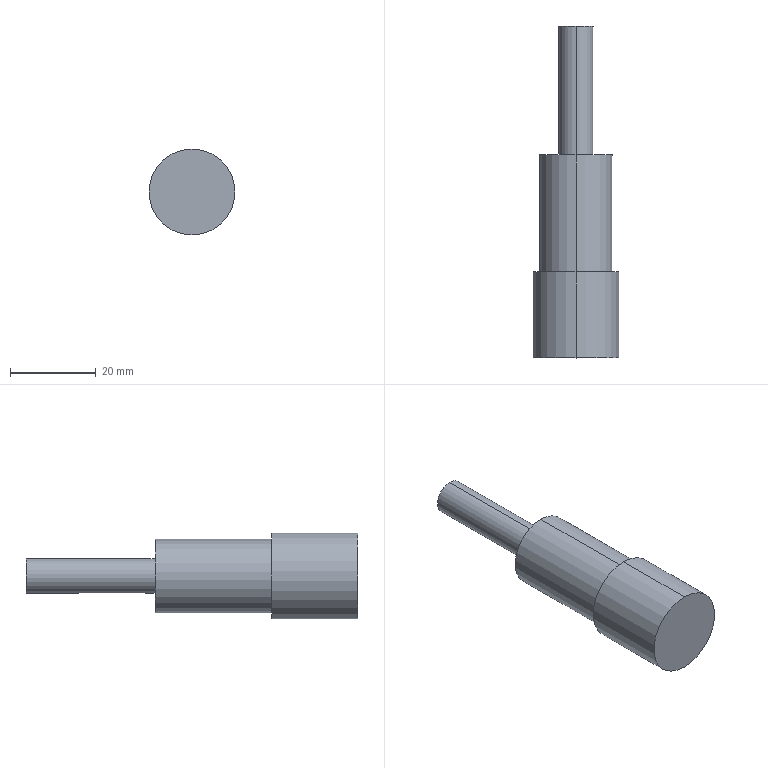Part | SolidWorks | features ICE 3, Extrusion 1 | 1 solid | 15 faces | box 20 x 77.2 x 20 mm | volume 13929 mm3 | cylinder 8 | plane 7 | commonest cylinder face diameters 2 x2 8 x2 17 x2 20 x2
STEP:
#1=CARTESIAN_POINT('',(0.,77.2,4.));
#2=VERTEX_POINT('',#1);
#3=CARTESIAN_POINT('',(0.,77.2,-4.));
#4=VERTEX_POINT('',#3);
#5=CARTESIAN_POINT('',(0.,77.2,0.));
#6=DIRECTION('',(0.,1.,0.));
#7=DIRECTION('',(0.,0.,1.));
#8=AXIS2_PLACEMENT_3D('',#5,#6,#7);
#9=CIRCLE('',#8,4.);
#10=EDGE_CURVE('',#2,#4,#9,.T.);
#11=ORIENTED_EDGE('',*,*,#10,.F.);
#12=CARTESIAN_POINT('',(0.,47.2,4.));
#13=VERTEX_POINT('',#12);
#14=CARTESIAN_POINT('',(0.,77.2,4.));
#15=DIRECTION('',(0.,-1.,0.));
#16=VECTOR('',#15,1000.);
#17=LINE('',#14,#16);
#18=EDGE_CURVE('',#2,#13,#17,.T.);
#19=ORIENTED_EDGE('',*,*,#18,.T.);
#20=CARTESIAN_POINT('',(0.,47.2,-4.));
#21=VERTEX_POINT('',#20);
#22=CARTESIAN_POINT('',(0.,47.2,0.));
#23=DIRECTION('',(0.,1.,0.));
#24=DIRECTION('',(0.,0.,1.));
#25=AXIS2_PLACEMENT_3D('',#22,#23,#24);
#26=CIRCLE('',#25,4.);
#27=EDGE_CURVE('',#13,#21,#26,.T.);
#28=ORIENTED_EDGE('',*,*,#27,.T.);
#29=CARTESIAN_POINT('',(0.,49.2,-4.));
#30=VERTEX_POINT('',#29);
#31=CARTESIAN_POINT('',(0.,77.2,-4.));
#32=DIRECTION('',(0.,-1.,0.));
#33=VECTOR('',#32,1000.);
#34=LINE('',#31,#33);
#35=EDGE_CURVE('',#30,#21,#34,.T.);
#36=ORIENTED_EDGE('',*,*,#35,.F.);
#37=CARTESIAN_POINT('',(1.,50.2,-3.873));
#38=VERTEX_POINT('',#37);
#39=CARTESIAN_POINT('',(0.,49.2,-4.));
#40=CARTESIAN_POINT('',(0.1309,49.2,-4.));
#41=CARTESIAN_POINT('',(0.2621,49.226,-3.993));
#42=CARTESIAN_POINT('',(0.5047,49.327,-3.97));
#43=CARTESIAN_POINT('',(0.6146,49.4,-3.954));
#44=CARTESIAN_POINT('',(0.7997,49.585,-3.92));
#45=CARTESIAN_POINT('',(0.8733,49.696,-3.904));
#46=CARTESIAN_POINT('',(0.9735,49.937,-3.88));
#47=CARTESIAN_POINT('',(1.,50.067,-3.873));
#48=CARTESIAN_POINT('',(1.,50.2,-3.873));
#49=B_SPLINE_CURVE_WITH_KNOTS('',3,(#39,#40,#41,#42,#43,#44,#45,#46,#47,#48),.UNSPECIFIED.,.F.,.F.,(4,2,2,2,4),(0.00157,0.001962,0.002354,0.002746,0.003138),.UNSPECIFIED.);
#50=EDGE_CURVE('',#30,#38,#49,.T.);
#51=ORIENTED_EDGE('',*,*,#50,.T.);
#52=CARTESIAN_POINT('',(1.,64.2,-3.873));
#53=VERTEX_POINT('',#52);
#54=CARTESIAN_POINT('',(1.,77.2,-3.873));
#55=DIRECTION('',(0.,1.,0.));
#56=VECTOR('',#55,1000.);
#57=LINE('',#54,#56);
#58=EDGE_CURVE('',#38,#53,#57,.T.);
#59=ORIENTED_EDGE('',*,*,#58,.T.);
#60=CARTESIAN_POINT('',(0.,65.2,-4.));
#61=VERTEX_POINT('',#60);
#62=CARTESIAN_POINT('',(1.,64.2,-3.873));
#63=CARTESIAN_POINT('',(1.,64.333,-3.873));
#64=CARTESIAN_POINT('',(0.9737,64.463,-3.88));
#65=CARTESIAN_POINT('',(0.873,64.705,-3.904));
#66=CARTESIAN_POINT('',(0.7987,64.816,-3.921));
#67=CARTESIAN_POINT('',(0.6149,64.999,-3.954));
#68=CARTESIAN_POINT('',(0.5037,65.074,-3.97));
#69=CARTESIAN_POINT('',(0.2631,65.174,-3.993));
#70=CARTESIAN_POINT('',(0.1311,65.2,-4.));
#71=CARTESIAN_POINT('',(0.,65.2,-4.));
#72=B_SPLINE_CURVE_WITH_KNOTS('',3,(#62,#63,#64,#65,#66,#67,#68,#69,#70,#71),.UNSPECIFIED.,.F.,.F.,(4,2,2,2,4),(0.,0.0003925,0.0007849,0.001177,0.00157),.UNSPECIFIED.);
#73=EDGE_CURVE('',#53,#61,#72,.T.);
#74=ORIENTED_EDGE('',*,*,#73,.T.);
#75=CARTESIAN_POINT('',(0.,77.2,-4.));
#76=DIRECTION('',(0.,-1.,0.));
#77=VECTOR('',#76,1000.);
#78=LINE('',#75,#77);
#79=EDGE_CURVE('',#4,#61,#78,.T.);
#80=ORIENTED_EDGE('',*,*,#79,.F.);
#81=EDGE_LOOP('',(#11,#19,#28,#36,#51,#59,#74,#80));
#82=FACE_OUTER_BOUND('',#81,.T.);
#83=CARTESIAN_POINT('',(0.,77.2,0.));
#84=DIRECTION('',(0.,-1.,0.));
#85=DIRECTION('',(0.,0.,-1.));
#86=AXIS2_PLACEMENT_3D('',#83,#84,#85);
#87=CYLINDRICAL_SURFACE('',#86,4.);
#88=ADVANCED_FACE('',(#82),#87,.T.);
#89=CARTESIAN_POINT('',(0.,47.2,8.5));
#90=VERTEX_POINT('',#89);
#91=CARTESIAN_POINT('',(0.,47.2,-8.5));
#92=VERTEX_POINT('',#91);
#93=CARTESIAN_POINT('',(0.,47.2,0.));
#94=DIRECTION('',(0.,1.,0.));
#95=DIRECTION('',(0.,0.,1.));
#96=AXIS2_PLACEMENT_3D('',#93,#94,#95);
#97=CIRCLE('',#96,8.5);
#98=EDGE_CURVE('',#90,#92,#97,.T.);
#99=ORIENTED_EDGE('',*,*,#98,.F.);
#100=CARTESIAN_POINT('',(0.,20.,8.5));
#101=VERTEX_POINT('',#100);
#102=CARTESIAN_POINT('',(0.,47.2,8.5));
#103=DIRECTION('',(0.,-1.,0.));
#104=VECTOR('',#103,1000.);
#105=LINE('',#102,#104);
#106=EDGE_CURVE('',#90,#101,#105,.T.);
#107=ORIENTED_EDGE('',*,*,#106,.T.);
#108=CARTESIAN_POINT('',(0.,20.,-8.5));
#109=VERTEX_POINT('',#108);
#110=CARTESIAN_POINT('',(0.,20.,0.));
#111=DIRECTION('',(0.,1.,0.));
#112=DIRECTION('',(0.,0.,1.));
#113=AXIS2_PLACEMENT_3D('',#110,#111,#112);
#114=CIRCLE('',#113,8.5);
#115=EDGE_CURVE('',#101,#109,#114,.T.);
#116=ORIENTED_EDGE('',*,*,#115,.T.);
#117=CARTESIAN_POINT('',(0.,47.2,-8.5));
#118=DIRECTION('',(0.,-1.,0.));
#119=VECTOR('',#118,1000.);
#120=LINE('',#117,#119);
#121=EDGE_CURVE('',#92,#109,#120,.T.);
#122=ORIENTED_EDGE('',*,*,#121,.F.);
#123=EDGE_LOOP('',(#99,#107,#116,#122));
#124=FACE_OUTER_BOUND('',#123,.T.);
#125=CARTESIAN_POINT('',(0.,47.2,0.));
#126=DIRECTION('',(0.,-1.,0.));
#127=DIRECTION('',(0.,0.,-1.));
#128=AXIS2_PLACEMENT_3D('',#125,#126,#127);
#129=CYLINDRICAL_SURFACE('',#128,8.5);
#130=ADVANCED_FACE('',(#124),#129,.T.);
#131=CARTESIAN_POINT('',(0.,20.,10.));
#132=VERTEX_POINT('',#131);
#133=CARTESIAN_POINT('',(0.,20.,-10.));
#134=VERTEX_POINT('',#133);
#135=CARTESIAN_POINT('',(0.,20.,0.));
#136=DIRECTION('',(0.,1.,0.));
#137=DIRECTION('',(0.,0.,1.));
#138=AXIS2_PLACEMENT_3D('',#135,#136,#137);
#139=CIRCLE('',#138,10.);
#140=EDGE_CURVE('',#132,#134,#139,.T.);
#141=ORIENTED_EDGE('',*,*,#140,.F.);
#142=CARTESIAN_POINT('',(0.,0.,10.));
#143=VERTEX_POINT('',#142);
#144=CARTESIAN_POINT('',(0.,20.,10.));
#145=DIRECTION('',(0.,-1.,0.));
#146=VECTOR('',#145,1000.);
#147=LINE('',#144,#146);
#148=EDGE_CURVE('',#132,#143,#147,.T.);
#149=ORIENTED_EDGE('',*,*,#148,.T.);
#150=CARTESIAN_POINT('',(0.,0.,-10.));
#151=VERTEX_POINT('',#150);
#152=CARTESIAN_POINT('',(0.,0.,0.));
#153=DIRECTION('',(0.,1.,0.));
#154=DIRECTION('',(0.,0.,1.));
#155=AXIS2_PLACEMENT_3D('',#152,#153,#154);
#156=CIRCLE('',#155,10.);
#157=EDGE_CURVE('',#143,#151,#156,.T.);
#158=ORIENTED_EDGE('',*,*,#157,.T.);
#159=CARTESIAN_POINT('',(0.,20.,-10.));
#160=DIRECTION('',(0.,-1.,0.));
#161=VECTOR('',#160,1000.);
#162=LINE('',#159,#161);
#163=EDGE_CURVE('',#134,#151,#162,.T.);
#164=ORIENTED_EDGE('',*,*,#163,.F.);
#165=EDGE_LOOP('',(#141,#149,#158,#164));
#166=FACE_OUTER_BOUND('',#165,.T.);
#167=CARTESIAN_POINT('',(0.,20.,0.));
#168=DIRECTION('',(0.,-1.,0.));
#169=DIRECTION('',(0.,0.,-1.));
#170=AXIS2_PLACEMENT_3D('',#167,#168,#169);
#171=CYLINDRICAL_SURFACE('',#170,10.);
#172=ADVANCED_FACE('',(#166),#171,.T.);
#173=ORIENTED_EDGE('',*,*,#148,.F.);
#174=CARTESIAN_POINT('',(0.,20.,0.));
#175=DIRECTION('',(0.,1.,0.));
#176=DIRECTION('',(0.,0.,1.));
#177=AXIS2_PLACEMENT_3D('',#174,#175,#176);
#178=CIRCLE('',#177,10.);
#179=EDGE_CURVE('',#134,#132,#178,.T.);
#180=ORIENTED_EDGE('',*,*,#179,.F.);
#181=ORIENTED_EDGE('',*,*,#163,.T.);
#182=CARTESIAN_POINT('',(0.,0.,0.));
#183=DIRECTION('',(0.,1.,0.));
#184=DIRECTION('',(0.,0.,1.));
#185=AXIS2_PLACEMENT_3D('',#182,#183,#184);
#186=CIRCLE('',#185,10.);
#187=EDGE_CURVE('',#151,#143,#186,.T.);
#188=ORIENTED_EDGE('',*,*,#187,.T.);
#189=EDGE_LOOP('',(#173,#180,#181,#188));
#190=FACE_OUTER_BOUND('',#189,.T.);
#191=CARTESIAN_POINT('',(0.,20.,0.));
#192=DIRECTION('',(0.,-1.,0.));
#193=DIRECTION('',(0.,0.,-1.));
#194=AXIS2_PLACEMENT_3D('',#191,#192,#193);
#195=CYLINDRICAL_SURFACE('',#194,10.);
#196=ADVANCED_FACE('',(#190),#195,.T.);
#197=CARTESIAN_POINT('',(0.,20.,0.));
#198=DIRECTION('',(0.,1.,0.));
#199=DIRECTION('',(0.,0.,1.));
#200=AXIS2_PLACEMENT_3D('',#197,#198,#199);
#201=CIRCLE('',#200,8.5);
#202=EDGE_CURVE('',#109,#101,#201,.T.);
#203=ORIENTED_EDGE('',*,*,#202,.F.);
#204=ORIENTED_EDGE('',*,*,#115,.F.);
#205=EDGE_LOOP('',(#203,#204));
#206=FACE_BOUND('',#205,.T.);
#207=ORIENTED_EDGE('',*,*,#179,.T.);
#208=ORIENTED_EDGE('',*,*,#140,.T.);
#209=EDGE_LOOP('',(#207,#208));
#210=FACE_OUTER_BOUND('',#209,.T.);
#211=CARTESIAN_POINT('',(0.,20.,0.));
#212=DIRECTION('',(0.,1.,0.));
#213=DIRECTION('',(0.,0.,1.));
#214=AXIS2_PLACEMENT_3D('',#211,#212,#213);
#215=PLANE('',#214);
#216=ADVANCED_FACE('',(#206,#210),#215,.T.);
#217=ORIENTED_EDGE('',*,*,#187,.F.);
#218=ORIENTED_EDGE('',*,*,#157,.F.);
#219=EDGE_LOOP('',(#217,#218));
#220=FACE_OUTER_BOUND('',#219,.T.);
#221=CARTESIAN_POINT('',(0.,0.,0.));
#222=DIRECTION('',(0.,1.,0.));
#223=DIRECTION('',(0.,0.,1.));
#224=AXIS2_PLACEMENT_3D('',#221,#222,#223);
#225=PLANE('',#224);
#226=ADVANCED_FACE('',(#220),#225,.F.);
#227=ORIENTED_EDGE('',*,*,#106,.F.);
#228=CARTESIAN_POINT('',(0.,47.2,0.));
#229=DIRECTION('',(0.,1.,0.));
#230=DIRECTION('',(0.,0.,1.));
#231=AXIS2_PLACEMENT_3D('',#228,#229,#230);
#232=CIRCLE('',#231,8.5);
#233=EDGE_CURVE('',#92,#90,#232,.T.);
#234=ORIENTED_EDGE('',*,*,#233,.F.);
#235=ORIENTED_EDGE('',*,*,#121,.T.);
#236=ORIENTED_EDGE('',*,*,#202,.T.);
#237=EDGE_LOOP('',(#227,#234,#235,#236));
#238=FACE_OUTER_BOUND('',#237,.T.);
#239=CARTESIAN_POINT('',(0.,47.2,0.));
#240=DIRECTION('',(0.,-1.,0.));
#241=DIRECTION('',(0.,0.,-1.));
#242=AXIS2_PLACEMENT_3D('',#239,#240,#241);
#243=CYLINDRICAL_SURFACE('',#242,8.5);
#244=ADVANCED_FACE('',(#238),#243,.T.);
#245=CARTESIAN_POINT('',(0.,47.2,0.));
#246=DIRECTION('',(0.,1.,0.));
#247=DIRECTION('',(0.,0.,1.));
#248=AXIS2_PLACEMENT_3D('',#245,#246,#247);
#249=CIRCLE('',#248,4.);
#250=EDGE_CURVE('',#21,#13,#249,.T.);
#251=ORIENTED_EDGE('',*,*,#250,.F.);
#252=ORIENTED_EDGE('',*,*,#27,.F.);
#253=EDGE_LOOP('',(#251,#252));
#254=FACE_BOUND('',#253,.T.);
#255=ORIENTED_EDGE('',*,*,#233,.T.);
#256=ORIENTED_EDGE('',*,*,#98,.T.);
#257=EDGE_LOOP('',(#255,#256));
#258=FACE_OUTER_BOUND('',#257,.T.);
#259=CARTESIAN_POINT('',(0.,47.2,0.));
#260=DIRECTION('',(0.,1.,0.));
#261=DIRECTION('',(0.,0.,1.));
#262=AXIS2_PLACEMENT_3D('',#259,#260,#261);
#263=PLANE('',#262);
#264=ADVANCED_FACE('',(#254,#258),#263,.T.);
#265=ORIENTED_EDGE('',*,*,#18,.F.);
#266=CARTESIAN_POINT('',(0.,77.2,0.));
#267=DIRECTION('',(0.,1.,0.));
#268=DIRECTION('',(0.,0.,1.));
#269=AXIS2_PLACEMENT_3D('',#266,#267,#268);
#270=CIRCLE('',#269,4.);
#271=EDGE_CURVE('',#4,#2,#270,.T.);
#272=ORIENTED_EDGE('',*,*,#271,.F.);
#273=ORIENTED_EDGE('',*,*,#79,.T.);
#274=CARTESIAN_POINT('',(-1.,64.2,-3.873));
#275=VERTEX_POINT('',#274);
#276=CARTESIAN_POINT('',(0.,65.2,-4.));
#277=CARTESIAN_POINT('',(-0.1309,65.2,-4.));
#278=CARTESIAN_POINT('',(-0.2621,65.174,-3.993));
#279=CARTESIAN_POINT('',(-0.5047,65.073,-3.97));
#280=CARTESIAN_POINT('',(-0.6146,65.,-3.954));
#281=CARTESIAN_POINT('',(-0.7997,64.815,-3.92));
#282=CARTESIAN_POINT('',(-0.8733,64.704,-3.904));
#283=CARTESIAN_POINT('',(-0.9735,64.463,-3.88));
#284=CARTESIAN_POINT('',(-1.,64.333,-3.873));
#285=CARTESIAN_POINT('',(-1.,64.2,-3.873));
#286=B_SPLINE_CURVE_WITH_KNOTS('',3,(#276,#277,#278,#279,#280,#281,#282,#283,#284,#285),.UNSPECIFIED.,.F.,.F.,(4,2,2,2,4),(0.00157,0.001962,0.002354,0.002746,0.003138),.UNSPECIFIED.);
#287=EDGE_CURVE('',#61,#275,#286,.T.);
#288=ORIENTED_EDGE('',*,*,#287,.T.);
#289=CARTESIAN_POINT('',(-1.,50.2,-3.873));
#290=VERTEX_POINT('',#289);
#291=CARTESIAN_POINT('',(-1.,77.2,-3.873));
#292=DIRECTION('',(0.,-1.,0.));
#293=VECTOR('',#292,1000.);
#294=LINE('',#291,#293);
#295=EDGE_CURVE('',#275,#290,#294,.T.);
#296=ORIENTED_EDGE('',*,*,#295,.T.);
#297=CARTESIAN_POINT('',(-1.,50.2,-3.873));
#298=CARTESIAN_POINT('',(-1.,50.067,-3.873));
#299=CARTESIAN_POINT('',(-0.9737,49.937,-3.88));
#300=CARTESIAN_POINT('',(-0.873,49.695,-3.904));
#301=CARTESIAN_POINT('',(-0.7987,49.584,-3.921));
#302=CARTESIAN_POINT('',(-0.6149,49.401,-3.954));
#303=CARTESIAN_POINT('',(-0.5037,49.326,-3.97));
#304=CARTESIAN_POINT('',(-0.2631,49.226,-3.993));
#305=CARTESIAN_POINT('',(-0.1311,49.2,-4.));
#306=CARTESIAN_POINT('',(0.,49.2,-4.));
#307=B_SPLINE_CURVE_WITH_KNOTS('',3,(#297,#298,#299,#300,#301,#302,#303,#304,#305,#306),.UNSPECIFIED.,.F.,.F.,(4,2,2,2,4),(0.,0.0003925,0.0007849,0.001177,0.00157),.UNSPECIFIED.);
#308=EDGE_CURVE('',#290,#30,#307,.T.);
#309=ORIENTED_EDGE('',*,*,#308,.T.);
#310=ORIENTED_EDGE('',*,*,#35,.T.);
#311=ORIENTED_EDGE('',*,*,#250,.T.);
#312=EDGE_LOOP('',(#265,#272,#273,#288,#296,#309,#310,#311));
#313=FACE_OUTER_BOUND('',#312,.T.);
#314=CARTESIAN_POINT('',(0.,77.2,0.));
#315=DIRECTION('',(0.,-1.,0.));
#316=DIRECTION('',(0.,0.,-1.));
#317=AXIS2_PLACEMENT_3D('',#314,#315,#316);
#318=CYLINDRICAL_SURFACE('',#317,4.);
#319=ADVANCED_FACE('',(#313),#318,.T.);
#320=ORIENTED_EDGE('',*,*,#271,.T.);
#321=ORIENTED_EDGE('',*,*,#10,.T.);
#322=EDGE_LOOP('',(#320,#321));
#323=FACE_OUTER_BOUND('',#322,.T.);
#324=CARTESIAN_POINT('',(0.,77.2,0.));
#325=DIRECTION('',(0.,1.,0.));
#326=DIRECTION('',(0.,0.,1.));
#327=AXIS2_PLACEMENT_3D('',#324,#325,#326);
#328=PLANE('',#327);
#329=ADVANCED_FACE('',(#323),#328,.T.);
#330=CARTESIAN_POINT('',(-1.,50.2,-2.8));
#331=VERTEX_POINT('',#330);
#332=CARTESIAN_POINT('',(-1.,50.2,-2.8));
#333=DIRECTION('',(0.,0.,-1.));
#334=VECTOR('',#333,1000.);
#335=LINE('',#332,#334);
#336=EDGE_CURVE('',#331,#290,#335,.T.);
#337=ORIENTED_EDGE('',*,*,#336,.F.);
#338=CARTESIAN_POINT('',(1.,50.2,-2.8));
#339=VERTEX_POINT('',#338);
#340=CARTESIAN_POINT('',(0.,50.2,-2.8));
#341=DIRECTION('',(0.,0.,-1.));
#342=DIRECTION('',(-1.,0.,0.));
#343=AXIS2_PLACEMENT_3D('',#340,#341,#342);
#344=CIRCLE('',#343,1.);
#345=EDGE_CURVE('',#339,#331,#344,.T.);
#346=ORIENTED_EDGE('',*,*,#345,.F.);
#347=CARTESIAN_POINT('',(1.,50.2,-2.8));
#348=DIRECTION('',(0.,0.,-1.));
#349=VECTOR('',#348,1000.);
#350=LINE('',#347,#349);
#351=EDGE_CURVE('',#339,#38,#350,.T.);
#352=ORIENTED_EDGE('',*,*,#351,.T.);
#353=ORIENTED_EDGE('',*,*,#50,.F.);
#354=ORIENTED_EDGE('',*,*,#308,.F.);
#355=EDGE_LOOP('',(#337,#346,#352,#353,#354));
#356=FACE_OUTER_BOUND('',#355,.T.);
#357=CARTESIAN_POINT('',(0.,50.2,-2.8));
#358=DIRECTION('',(0.,0.,-1.));
#359=DIRECTION('',(-1.,0.,0.));
#360=AXIS2_PLACEMENT_3D('',#357,#358,#359);
#361=CYLINDRICAL_SURFACE('',#360,1.);
#362=ADVANCED_FACE('',(#356),#361,.F.);
#363=ORIENTED_EDGE('',*,*,#351,.F.);
#364=CARTESIAN_POINT('',(1.,64.2,-2.8));
#365=VERTEX_POINT('',#364);
#366=CARTESIAN_POINT('',(1.,50.2,-2.8));
#367=DIRECTION('',(0.,-1.,0.));
#368=VECTOR('',#367,1000.);
#369=LINE('',#366,#368);
#370=EDGE_CURVE('',#365,#339,#369,.T.);
#371=ORIENTED_EDGE('',*,*,#370,.F.);
#372=CARTESIAN_POINT('',(1.,64.2,-2.8));
#373=DIRECTION('',(0.,0.,-1.));
#374=VECTOR('',#373,1000.);
#375=LINE('',#372,#374);
#376=EDGE_CURVE('',#365,#53,#375,.T.);
#377=ORIENTED_EDGE('',*,*,#376,.T.);
#378=ORIENTED_EDGE('',*,*,#58,.F.);
#379=EDGE_LOOP('',(#363,#371,#377,#378));
#380=FACE_OUTER_BOUND('',#379,.T.);
#381=CARTESIAN_POINT('',(1.,50.2,-2.8));
#382=DIRECTION('',(1.,0.,0.));
#383=DIRECTION('',(0.,0.,-1.));
#384=AXIS2_PLACEMENT_3D('',#381,#382,#383);
#385=PLANE('',#384);
#386=ADVANCED_FACE('',(#380),#385,.F.);
#387=ORIENTED_EDGE('',*,*,#376,.F.);
#388=CARTESIAN_POINT('',(-1.,64.2,-2.8));
#389=VERTEX_POINT('',#388);
#390=CARTESIAN_POINT('',(0.,64.2,-2.8));
#391=DIRECTION('',(0.,0.,-1.));
#392=DIRECTION('',(-1.,0.,0.));
#393=AXIS2_PLACEMENT_3D('',#390,#391,#392);
#394=CIRCLE('',#393,1.);
#395=EDGE_CURVE('',#389,#365,#394,.T.);
#396=ORIENTED_EDGE('',*,*,#395,.F.);
#397=CARTESIAN_POINT('',(-1.,64.2,-2.8));
#398=DIRECTION('',(0.,0.,-1.));
#399=VECTOR('',#398,1000.);
#400=LINE('',#397,#399);
#401=EDGE_CURVE('',#389,#275,#400,.T.);
#402=ORIENTED_EDGE('',*,*,#401,.T.);
#403=ORIENTED_EDGE('',*,*,#287,.F.);
#404=ORIENTED_EDGE('',*,*,#73,.F.);
#405=EDGE_LOOP('',(#387,#396,#402,#403,#404));
#406=FACE_OUTER_BOUND('',#405,.T.);
#407=CARTESIAN_POINT('',(0.,64.2,-2.8));
#408=DIRECTION('',(0.,0.,-1.));
#409=DIRECTION('',(-1.,0.,0.));
#410=AXIS2_PLACEMENT_3D('',#407,#408,#409);
#411=CYLINDRICAL_SURFACE('',#410,1.);
#412=ADVANCED_FACE('',(#406),#411,.F.);
#413=ORIENTED_EDGE('',*,*,#401,.F.);
#414=CARTESIAN_POINT('',(-1.,50.2,-2.8));
#415=DIRECTION('',(0.,1.,0.));
#416=VECTOR('',#415,1000.);
#417=LINE('',#414,#416);
#418=EDGE_CURVE('',#331,#389,#417,.T.);
#419=ORIENTED_EDGE('',*,*,#418,.F.);
#420=ORIENTED_EDGE('',*,*,#336,.T.);
#421=ORIENTED_EDGE('',*,*,#295,.F.);
#422=EDGE_LOOP('',(#413,#419,#420,#421));
#423=FACE_OUTER_BOUND('',#422,.T.);
#424=CARTESIAN_POINT('',(-1.,50.2,-2.8));
#425=DIRECTION('',(-1.,0.,0.));
#426=DIRECTION('',(0.,0.,1.));
#427=AXIS2_PLACEMENT_3D('',#424,#425,#426);
#428=PLANE('',#427);
#429=ADVANCED_FACE('',(#423),#428,.F.);
#430=ORIENTED_EDGE('',*,*,#345,.T.);
#431=ORIENTED_EDGE('',*,*,#418,.T.);
#432=ORIENTED_EDGE('',*,*,#395,.T.);
#433=ORIENTED_EDGE('',*,*,#370,.T.);
#434=EDGE_LOOP('',(#430,#431,#432,#433));
#435=FACE_OUTER_BOUND('',#434,.T.);
#436=CARTESIAN_POINT('',(0.,50.2,-2.8));
#437=DIRECTION('',(0.,0.,-1.));
#438=DIRECTION('',(-1.,0.,0.));
#439=AXIS2_PLACEMENT_3D('',#436,#437,#438);
#440=PLANE('',#439);
#441=ADVANCED_FACE('',(#435),#440,.T.);
#442=CLOSED_SHELL('',(#88,#130,#172,#196,#216,#226,#244,#264,#319,#329,#362,#386,#412,#429,#441));
#443=MANIFOLD_SOLID_BREP('',#442);
#444=CARTESIAN_POINT('',(0.,0.,0.));
#445=DIRECTION('',(0.,0.,1.));
#446=DIRECTION('',(1.,0.,0.));
#447=AXIS2_PLACEMENT_3D('',#444,#445,#446);
#448=(LENGTH_UNIT()NAMED_UNIT(*)SI_UNIT(.MILLI.,.METRE.));
#449=UNCERTAINTY_MEASURE_WITH_UNIT(LENGTH_MEASURE(0.00001),#448,'','');
#450=(NAMED_UNIT(*)PLANE_ANGLE_UNIT()SI_UNIT($,.RADIAN.));
#451=(NAMED_UNIT(*)SI_UNIT($,.STERADIAN.)SOLID_ANGLE_UNIT());
#452=(GEOMETRIC_REPRESENTATION_CONTEXT(3)GLOBAL_UNCERTAINTY_ASSIGNED_CONTEXT((#449))GLOBAL_UNIT_ASSIGNED_CONTEXT((#448,#450,#451))REPRESENTATION_CONTEXT('',''));
#453=ADVANCED_BREP_SHAPE_REPRESENTATION('',(#443,#447),#452);